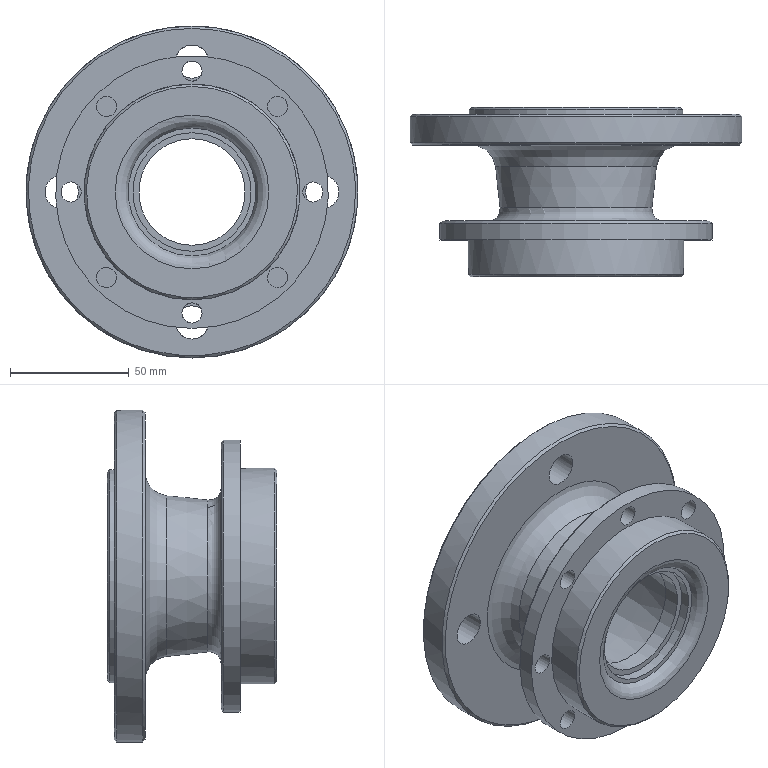Part | NX | features DATUM_CSYS 4, SKETCH 3, EXTRUDE 2, BLEND 1, CHAMFER 1, SWP104 1 | 1 solid | 37 faces | box 140 x 71.5 x 140 mm | volume 362768 mm3 | cylinder 19 | plane 8 | cone 7 | torus 3 | commonest cylinder face diameters 8.5 x8 14 x4 45 x1 50 x1 54 x1 90 x1
STEP:
#1=CARTESIAN_POINT('',(0.,0.,32.408));
#2=VERTEX_POINT('',#1);
#3=CARTESIAN_POINT('',(0.,0.,0.));
#4=DIRECTION('',(0.,1.,0.));
#5=DIRECTION('',(0.,0.,1.));
#6=AXIS2_PLACEMENT_3D('',#3,#4,#5);
#7=CIRCLE('',#6,32.408);
#8=EDGE_CURVE('',#2,#2,#7,.T.);
#9=ORIENTED_EDGE('',*,*,#8,.T.);
#10=EDGE_LOOP('',(#9));
#11=FACE_BOUND('',#10,.T.);
#12=CARTESIAN_POINT('',(0.,0.,44.5));
#13=VERTEX_POINT('',#12);
#14=CARTESIAN_POINT('',(0.,0.,0.));
#15=DIRECTION('',(0.,1.,0.));
#16=DIRECTION('',(0.,0.,1.));
#17=AXIS2_PLACEMENT_3D('',#14,#15,#16);
#18=CIRCLE('',#17,44.5);
#19=EDGE_CURVE('',#13,#13,#18,.F.);
#20=ORIENTED_EDGE('',*,*,#19,.T.);
#21=EDGE_LOOP('',(#20));
#22=FACE_BOUND('',#21,.T.);
#23=CARTESIAN_POINT('',(0.,0.,45.5));
#24=DIRECTION('',(0.,1.,0.));
#25=DIRECTION('',(0.,0.,1.));
#26=AXIS2_PLACEMENT_3D('',#23,#24,#25);
#27=PLANE('',#26);
#28=ADVANCED_FACE('',(#11,#22),#27,.F.);
#29=CARTESIAN_POINT('',(0.,4.5,-25.));
#30=VERTEX_POINT('',#29);
#31=CARTESIAN_POINT('',(0.,4.5,0.));
#32=DIRECTION('',(0.,-1.,0.));
#33=DIRECTION('',(0.,0.,-1.));
#34=AXIS2_PLACEMENT_3D('',#31,#32,#33);
#35=CIRCLE('',#34,25.);
#36=EDGE_CURVE('',#30,#30,#35,.T.);
#37=ORIENTED_EDGE('',*,*,#36,.F.);
#38=EDGE_LOOP('',(#37));
#39=FACE_BOUND('',#38,.T.);
#40=CARTESIAN_POINT('',(0.,4.5,-27.));
#41=VERTEX_POINT('',#40);
#42=CARTESIAN_POINT('',(0.,4.5,0.));
#43=DIRECTION('',(0.,-1.,0.));
#44=DIRECTION('',(0.,0.,-1.));
#45=AXIS2_PLACEMENT_3D('',#42,#43,#44);
#46=CIRCLE('',#45,27.);
#47=EDGE_CURVE('',#41,#41,#46,.T.);
#48=ORIENTED_EDGE('',*,*,#47,.T.);
#49=EDGE_LOOP('',(#48));
#50=FACE_BOUND('',#49,.T.);
#51=CARTESIAN_POINT('',(0.,4.5,27.));
#52=DIRECTION('',(0.,1.,0.));
#53=DIRECTION('',(0.,0.,1.));
#54=AXIS2_PLACEMENT_3D('',#51,#52,#53);
#55=PLANE('',#54);
#56=ADVANCED_FACE('',(#39,#50),#55,.F.);
#57=CARTESIAN_POINT('',(0.,8.5,-25.));
#58=VERTEX_POINT('',#57);
#59=CARTESIAN_POINT('',(0.,8.5,0.));
#60=DIRECTION('',(0.,-1.,0.));
#61=DIRECTION('',(0.,0.,-1.));
#62=AXIS2_PLACEMENT_3D('',#59,#60,#61);
#63=CIRCLE('',#62,25.);
#64=EDGE_CURVE('',#58,#58,#63,.T.);
#65=ORIENTED_EDGE('',*,*,#64,.F.);
#66=EDGE_LOOP('',(#65));
#67=FACE_BOUND('',#66,.T.);
#68=ORIENTED_EDGE('',*,*,#36,.T.);
#69=EDGE_LOOP('',(#68));
#70=FACE_BOUND('',#69,.T.);
#71=CARTESIAN_POINT('',(0.,0.,0.));
#72=DIRECTION('',(0.,-1.,0.));
#73=DIRECTION('',(0.,0.,-1.));
#74=AXIS2_PLACEMENT_3D('',#71,#72,#73);
#75=CYLINDRICAL_SURFACE('',#74,25.);
#76=ADVANCED_FACE('',(#67,#70),#75,.F.);
#77=CARTESIAN_POINT('',(0.,8.5,-22.5));
#78=VERTEX_POINT('',#77);
#79=CARTESIAN_POINT('',(0.,8.5,0.));
#80=DIRECTION('',(0.,-1.,0.));
#81=DIRECTION('',(0.,0.,-1.));
#82=AXIS2_PLACEMENT_3D('',#79,#80,#81);
#83=CIRCLE('',#82,22.5);
#84=EDGE_CURVE('',#78,#78,#83,.T.);
#85=ORIENTED_EDGE('',*,*,#84,.F.);
#86=EDGE_LOOP('',(#85));
#87=FACE_BOUND('',#86,.T.);
#88=ORIENTED_EDGE('',*,*,#64,.T.);
#89=EDGE_LOOP('',(#88));
#90=FACE_BOUND('',#89,.T.);
#91=CARTESIAN_POINT('',(0.,8.5,25.));
#92=DIRECTION('',(0.,1.,0.));
#93=DIRECTION('',(0.,0.,1.));
#94=AXIS2_PLACEMENT_3D('',#91,#92,#93);
#95=PLANE('',#94);
#96=ADVANCED_FACE('',(#87,#90),#95,.F.);
#97=CARTESIAN_POINT('',(0.,15.5,-22.5));
#98=VERTEX_POINT('',#97);
#99=CARTESIAN_POINT('',(0.,15.5,0.));
#100=DIRECTION('',(0.,-1.,0.));
#101=DIRECTION('',(0.,0.,-1.));
#102=AXIS2_PLACEMENT_3D('',#99,#100,#101);
#103=CIRCLE('',#102,22.5);
#104=EDGE_CURVE('',#98,#98,#103,.T.);
#105=ORIENTED_EDGE('',*,*,#104,.F.);
#106=EDGE_LOOP('',(#105));
#107=FACE_BOUND('',#106,.T.);
#108=ORIENTED_EDGE('',*,*,#84,.T.);
#109=EDGE_LOOP('',(#108));
#110=FACE_BOUND('',#109,.T.);
#111=CARTESIAN_POINT('',(0.,0.,0.));
#112=DIRECTION('',(0.,-1.,0.));
#113=DIRECTION('',(0.,0.,-1.));
#114=AXIS2_PLACEMENT_3D('',#111,#112,#113);
#115=CYLINDRICAL_SURFACE('',#114,22.5);
#116=ADVANCED_FACE('',(#107,#110),#115,.F.);
#117=CARTESIAN_POINT('',(0.,56.5,-27.));
#118=VERTEX_POINT('',#117);
#119=CARTESIAN_POINT('',(0.,56.5,0.));
#120=DIRECTION('',(0.,-1.,0.));
#121=DIRECTION('',(0.,0.,-1.));
#122=AXIS2_PLACEMENT_3D('',#119,#120,#121);
#123=CIRCLE('',#122,27.);
#124=EDGE_CURVE('',#118,#118,#123,.T.);
#125=ORIENTED_EDGE('',*,*,#124,.F.);
#126=EDGE_LOOP('',(#125));
#127=FACE_BOUND('',#126,.T.);
#128=ORIENTED_EDGE('',*,*,#104,.T.);
#129=EDGE_LOOP('',(#128));
#130=FACE_BOUND('',#129,.T.);
#131=CARTESIAN_POINT('',(0.,15.5,0.));
#132=DIRECTION('',(0.,1.,0.));
#133=DIRECTION('',(0.,0.,1.));
#134=AXIS2_PLACEMENT_3D('',#131,#132,#133);
#135=CONICAL_SURFACE('',#134,22.5,0.1093);
#136=ADVANCED_FACE('',(#127,#130),#135,.F.);
#137=CARTESIAN_POINT('',(0.,71.5,-27.));
#138=VERTEX_POINT('',#137);
#139=CARTESIAN_POINT('',(0.,71.5,0.));
#140=DIRECTION('',(0.,-1.,0.));
#141=DIRECTION('',(0.,0.,-1.));
#142=AXIS2_PLACEMENT_3D('',#139,#140,#141);
#143=CIRCLE('',#142,27.);
#144=EDGE_CURVE('',#138,#138,#143,.T.);
#145=ORIENTED_EDGE('',*,*,#144,.F.);
#146=EDGE_LOOP('',(#145));
#147=FACE_BOUND('',#146,.T.);
#148=ORIENTED_EDGE('',*,*,#124,.T.);
#149=EDGE_LOOP('',(#148));
#150=FACE_BOUND('',#149,.T.);
#151=CARTESIAN_POINT('',(0.,0.,0.));
#152=DIRECTION('',(0.,-1.,0.));
#153=DIRECTION('',(0.,0.,-1.));
#154=AXIS2_PLACEMENT_3D('',#151,#152,#153);
#155=CYLINDRICAL_SURFACE('',#154,27.);
#156=ADVANCED_FACE('',(#147,#150),#155,.F.);
#157=CARTESIAN_POINT('',(0.,71.5,-44.));
#158=VERTEX_POINT('',#157);
#159=CARTESIAN_POINT('',(0.,71.5,0.));
#160=DIRECTION('',(0.,-1.,0.));
#161=DIRECTION('',(0.,0.,-1.));
#162=AXIS2_PLACEMENT_3D('',#159,#160,#161);
#163=CIRCLE('',#162,44.);
#164=EDGE_CURVE('',#158,#158,#163,.F.);
#165=ORIENTED_EDGE('',*,*,#164,.T.);
#166=EDGE_LOOP('',(#165));
#167=FACE_BOUND('',#166,.T.);
#168=ORIENTED_EDGE('',*,*,#144,.T.);
#169=EDGE_LOOP('',(#168));
#170=FACE_BOUND('',#169,.T.);
#171=CARTESIAN_POINT('',(0.,71.5,27.));
#172=DIRECTION('',(0.,-1.,0.));
#173=DIRECTION('',(0.,0.,-1.));
#174=AXIS2_PLACEMENT_3D('',#171,#172,#173);
#175=PLANE('',#174);
#176=ADVANCED_FACE('',(#167,#170),#175,.F.);
#177=CARTESIAN_POINT('',(0.,70.5,-45.));
#178=VERTEX_POINT('',#177);
#179=CARTESIAN_POINT('',(0.,70.5,0.));
#180=DIRECTION('',(0.,-1.,0.));
#181=DIRECTION('',(0.,0.,-1.));
#182=AXIS2_PLACEMENT_3D('',#179,#180,#181);
#183=CIRCLE('',#182,45.);
#184=EDGE_CURVE('',#178,#178,#183,.T.);
#185=ORIENTED_EDGE('',*,*,#184,.T.);
#186=EDGE_LOOP('',(#185));
#187=FACE_BOUND('',#186,.T.);
#188=CARTESIAN_POINT('',(0.,68.5,-45.));
#189=VERTEX_POINT('',#188);
#190=CARTESIAN_POINT('',(0.,68.5,0.));
#191=DIRECTION('',(0.,-1.,0.));
#192=DIRECTION('',(0.,0.,-1.));
#193=AXIS2_PLACEMENT_3D('',#190,#191,#192);
#194=CIRCLE('',#193,45.);
#195=EDGE_CURVE('',#189,#189,#194,.T.);
#196=ORIENTED_EDGE('',*,*,#195,.F.);
#197=EDGE_LOOP('',(#196));
#198=FACE_BOUND('',#197,.T.);
#199=CARTESIAN_POINT('',(0.,0.,0.));
#200=DIRECTION('',(0.,-1.,0.));
#201=DIRECTION('',(0.,0.,-1.));
#202=AXIS2_PLACEMENT_3D('',#199,#200,#201);
#203=CYLINDRICAL_SURFACE('',#202,45.);
#204=ADVANCED_FACE('',(#187,#198),#203,.T.);
#205=CARTESIAN_POINT('',(55.,68.5,-7.));
#206=VERTEX_POINT('',#205);
#207=CARTESIAN_POINT('',(55.,68.5,0.));
#208=DIRECTION('',(0.,-1.,0.));
#209=DIRECTION('',(0.,0.,-1.));
#210=AXIS2_PLACEMENT_3D('',#207,#208,#209);
#211=CIRCLE('',#210,7.);
#212=EDGE_CURVE('',#206,#206,#211,.T.);
#213=ORIENTED_EDGE('',*,*,#212,.T.);
#214=EDGE_LOOP('',(#213));
#215=FACE_BOUND('',#214,.T.);
#216=CARTESIAN_POINT('',(0.,68.5,-62.));
#217=VERTEX_POINT('',#216);
#218=CARTESIAN_POINT('',(0.,68.5,-55.));
#219=DIRECTION('',(0.,-1.,0.));
#220=DIRECTION('',(0.,0.,-1.));
#221=AXIS2_PLACEMENT_3D('',#218,#219,#220);
#222=CIRCLE('',#221,7.);
#223=EDGE_CURVE('',#217,#217,#222,.T.);
#224=ORIENTED_EDGE('',*,*,#223,.T.);
#225=EDGE_LOOP('',(#224));
#226=FACE_BOUND('',#225,.T.);
#227=CARTESIAN_POINT('',(-55.,68.5,-7.));
#228=VERTEX_POINT('',#227);
#229=CARTESIAN_POINT('',(-55.,68.5,0.));
#230=DIRECTION('',(0.,-1.,0.));
#231=DIRECTION('',(0.,0.,-1.));
#232=AXIS2_PLACEMENT_3D('',#229,#230,#231);
#233=CIRCLE('',#232,7.);
#234=EDGE_CURVE('',#228,#228,#233,.T.);
#235=ORIENTED_EDGE('',*,*,#234,.T.);
#236=EDGE_LOOP('',(#235));
#237=FACE_BOUND('',#236,.T.);
#238=CARTESIAN_POINT('',(0.,68.5,48.));
#239=VERTEX_POINT('',#238);
#240=CARTESIAN_POINT('',(0.,68.5,55.));
#241=DIRECTION('',(0.,-1.,0.));
#242=DIRECTION('',(0.,0.,-1.));
#243=AXIS2_PLACEMENT_3D('',#240,#241,#242);
#244=CIRCLE('',#243,7.);
#245=EDGE_CURVE('',#239,#239,#244,.T.);
#246=ORIENTED_EDGE('',*,*,#245,.T.);
#247=EDGE_LOOP('',(#246));
#248=FACE_BOUND('',#247,.T.);
#249=CARTESIAN_POINT('',(0.,68.5,-69.));
#250=VERTEX_POINT('',#249);
#251=CARTESIAN_POINT('',(0.,68.5,0.));
#252=DIRECTION('',(0.,-1.,0.));
#253=DIRECTION('',(0.,0.,-1.));
#254=AXIS2_PLACEMENT_3D('',#251,#252,#253);
#255=CIRCLE('',#254,69.);
#256=EDGE_CURVE('',#250,#250,#255,.F.);
#257=ORIENTED_EDGE('',*,*,#256,.T.);
#258=EDGE_LOOP('',(#257));
#259=FACE_BOUND('',#258,.T.);
#260=ORIENTED_EDGE('',*,*,#195,.T.);
#261=EDGE_LOOP('',(#260));
#262=FACE_BOUND('',#261,.T.);
#263=CARTESIAN_POINT('',(0.,68.5,45.));
#264=DIRECTION('',(0.,-1.,0.));
#265=DIRECTION('',(0.,0.,-1.));
#266=AXIS2_PLACEMENT_3D('',#263,#264,#265);
#267=PLANE('',#266);
#268=ADVANCED_FACE('',(#215,#226,#237,#248,#259,#262),#267,.F.);
#269=CARTESIAN_POINT('',(0.,67.5,-70.));
#270=VERTEX_POINT('',#269);
#271=CARTESIAN_POINT('',(0.,67.5,0.));
#272=DIRECTION('',(0.,-1.,0.));
#273=DIRECTION('',(0.,0.,-1.));
#274=AXIS2_PLACEMENT_3D('',#271,#272,#273);
#275=CIRCLE('',#274,70.);
#276=EDGE_CURVE('',#270,#270,#275,.T.);
#277=ORIENTED_EDGE('',*,*,#276,.T.);
#278=EDGE_LOOP('',(#277));
#279=FACE_BOUND('',#278,.T.);
#280=CARTESIAN_POINT('',(0.,56.5,70.));
#281=VERTEX_POINT('',#280);
#282=CARTESIAN_POINT('',(0.,56.5,0.));
#283=DIRECTION('',(0.,1.,0.));
#284=DIRECTION('',(0.,0.,1.));
#285=AXIS2_PLACEMENT_3D('',#282,#283,#284);
#286=CIRCLE('',#285,70.);
#287=EDGE_CURVE('',#281,#281,#286,.T.);
#288=ORIENTED_EDGE('',*,*,#287,.T.);
#289=EDGE_LOOP('',(#288));
#290=FACE_BOUND('',#289,.T.);
#291=CARTESIAN_POINT('',(0.,0.,0.));
#292=DIRECTION('',(0.,-1.,0.));
#293=DIRECTION('',(0.,0.,-1.));
#294=AXIS2_PLACEMENT_3D('',#291,#292,#293);
#295=CYLINDRICAL_SURFACE('',#294,70.);
#296=ADVANCED_FACE('',(#279,#290),#295,.T.);
#297=CARTESIAN_POINT('',(55.,55.5,-7.));
#298=VERTEX_POINT('',#297);
#299=CARTESIAN_POINT('',(55.,55.5,0.));
#300=DIRECTION('',(0.,-1.,0.));
#301=DIRECTION('',(0.,0.,-1.));
#302=AXIS2_PLACEMENT_3D('',#299,#300,#301);
#303=CIRCLE('',#302,7.);
#304=EDGE_CURVE('',#298,#298,#303,.T.);
#305=ORIENTED_EDGE('',*,*,#304,.F.);
#306=EDGE_LOOP('',(#305));
#307=FACE_BOUND('',#306,.T.);
#308=CARTESIAN_POINT('',(-7.,55.5,-55.));
#309=VERTEX_POINT('',#308);
#310=CARTESIAN_POINT('',(0.,55.5,-55.));
#311=DIRECTION('',(0.,-1.,0.));
#312=DIRECTION('',(-1.,0.,0.));
#313=AXIS2_PLACEMENT_3D('',#310,#311,#312);
#314=CIRCLE('',#313,7.);
#315=EDGE_CURVE('',#309,#309,#314,.T.);
#316=ORIENTED_EDGE('',*,*,#315,.F.);
#317=EDGE_LOOP('',(#316));
#318=FACE_BOUND('',#317,.T.);
#319=CARTESIAN_POINT('',(-55.,55.5,7.));
#320=VERTEX_POINT('',#319);
#321=CARTESIAN_POINT('',(-55.,55.5,0.));
#322=DIRECTION('',(0.,-1.,0.));
#323=DIRECTION('',(0.,0.,1.));
#324=AXIS2_PLACEMENT_3D('',#321,#322,#323);
#325=CIRCLE('',#324,7.);
#326=EDGE_CURVE('',#320,#320,#325,.T.);
#327=ORIENTED_EDGE('',*,*,#326,.F.);
#328=EDGE_LOOP('',(#327));
#329=FACE_BOUND('',#328,.T.);
#330=CARTESIAN_POINT('',(7.,55.5,55.));
#331=VERTEX_POINT('',#330);
#332=CARTESIAN_POINT('',(0.,55.5,55.));
#333=DIRECTION('',(0.,-1.,0.));
#334=DIRECTION('',(1.,0.,0.));
#335=AXIS2_PLACEMENT_3D('',#332,#333,#334);
#336=CIRCLE('',#335,7.);
#337=EDGE_CURVE('',#331,#331,#336,.T.);
#338=ORIENTED_EDGE('',*,*,#337,.F.);
#339=EDGE_LOOP('',(#338));
#340=FACE_BOUND('',#339,.T.);
#341=CARTESIAN_POINT('',(0.,55.5,69.));
#342=VERTEX_POINT('',#341);
#343=CARTESIAN_POINT('',(0.,55.5,0.));
#344=DIRECTION('',(0.,1.,0.));
#345=DIRECTION('',(0.,0.,1.));
#346=AXIS2_PLACEMENT_3D('',#343,#344,#345);
#347=CIRCLE('',#346,69.);
#348=EDGE_CURVE('',#342,#342,#347,.F.);
#349=ORIENTED_EDGE('',*,*,#348,.T.);
#350=EDGE_LOOP('',(#349));
#351=FACE_BOUND('',#350,.T.);
#352=CARTESIAN_POINT('',(0.,55.5,-43.901));
#353=VERTEX_POINT('',#352);
#354=CARTESIAN_POINT('',(0.,55.5,0.));
#355=DIRECTION('',(0.,-1.,0.));
#356=DIRECTION('',(0.,0.,-1.));
#357=AXIS2_PLACEMENT_3D('',#354,#355,#356);
#358=CIRCLE('',#357,43.901);
#359=EDGE_CURVE('',#353,#353,#358,.T.);
#360=ORIENTED_EDGE('',*,*,#359,.F.);
#361=EDGE_LOOP('',(#360));
#362=FACE_BOUND('',#361,.T.);
#363=CARTESIAN_POINT('',(0.,55.5,70.));
#364=DIRECTION('',(0.,1.,0.));
#365=DIRECTION('',(0.,0.,1.));
#366=AXIS2_PLACEMENT_3D('',#363,#364,#365);
#367=PLANE('',#366);
#368=ADVANCED_FACE('',(#307,#318,#329,#340,#351,#362),#367,.F.);
#369=CARTESIAN_POINT('',(0.,46.591,-33.96));
#370=VERTEX_POINT('',#369);
#371=CARTESIAN_POINT('',(0.,46.591,0.));
#372=DIRECTION('',(0.,-1.,0.));
#373=DIRECTION('',(0.,0.,-1.));
#374=AXIS2_PLACEMENT_3D('',#371,#372,#373);
#375=CIRCLE('',#374,33.96);
#376=EDGE_CURVE('',#370,#370,#375,.T.);
#377=ORIENTED_EDGE('',*,*,#376,.F.);
#378=EDGE_LOOP('',(#377));
#379=FACE_BOUND('',#378,.T.);
#380=ORIENTED_EDGE('',*,*,#359,.T.);
#381=EDGE_LOOP('',(#380));
#382=FACE_BOUND('',#381,.T.);
#383=CARTESIAN_POINT('',(0.,45.5,0.));
#384=DIRECTION('',(0.,-1.,0.));
#385=DIRECTION('',(0.,0.,-1.));
#386=AXIS2_PLACEMENT_3D('',#383,#384,#385);
#387=TOROIDAL_SURFACE('',#386,43.901,10.);
#388=ADVANCED_FACE('',(#379,#382),#387,.F.);
#389=CARTESIAN_POINT('',(0.,29.046,-32.035));
#390=VERTEX_POINT('',#389);
#391=CARTESIAN_POINT('',(0.,29.046,0.));
#392=DIRECTION('',(0.,-1.,0.));
#393=DIRECTION('',(0.,0.,-1.));
#394=AXIS2_PLACEMENT_3D('',#391,#392,#393);
#395=CIRCLE('',#394,32.035);
#396=EDGE_CURVE('',#390,#390,#395,.T.);
#397=ORIENTED_EDGE('',*,*,#396,.F.);
#398=EDGE_LOOP('',(#397));
#399=FACE_BOUND('',#398,.T.);
#400=ORIENTED_EDGE('',*,*,#376,.T.);
#401=EDGE_LOOP('',(#400));
#402=FACE_BOUND('',#401,.T.);
#403=CARTESIAN_POINT('',(0.,46.591,0.));
#404=DIRECTION('',(0.,1.,0.));
#405=DIRECTION('',(0.,0.,1.));
#406=AXIS2_PLACEMENT_3D('',#403,#404,#405);
#407=CONICAL_SURFACE('',#406,33.96,0.1093);
#408=ADVANCED_FACE('',(#399,#402),#407,.T.);
#409=CARTESIAN_POINT('',(0.,23.5,-37.005));
#410=VERTEX_POINT('',#409);
#411=CARTESIAN_POINT('',(0.,23.5,0.));
#412=DIRECTION('',(0.,-1.,0.));
#413=DIRECTION('',(0.,0.,-1.));
#414=AXIS2_PLACEMENT_3D('',#411,#412,#413);
#415=CIRCLE('',#414,37.005);
#416=EDGE_CURVE('',#410,#410,#415,.T.);
#417=ORIENTED_EDGE('',*,*,#416,.F.);
#418=EDGE_LOOP('',(#417));
#419=FACE_BOUND('',#418,.T.);
#420=ORIENTED_EDGE('',*,*,#396,.T.);
#421=EDGE_LOOP('',(#420));
#422=FACE_BOUND('',#421,.T.);
#423=CARTESIAN_POINT('',(0.,28.5,0.));
#424=DIRECTION('',(0.,-1.,0.));
#425=DIRECTION('',(0.,0.,-1.));
#426=AXIS2_PLACEMENT_3D('',#423,#424,#425);
#427=TOROIDAL_SURFACE('',#426,37.005,5.);
#428=ADVANCED_FACE('',(#419,#422),#427,.F.);
#429=CARTESIAN_POINT('',(51.,23.5,-4.25));
#430=VERTEX_POINT('',#429);
#431=CARTESIAN_POINT('',(51.,23.5,0.));
#432=DIRECTION('',(0.,-1.,0.));
#433=DIRECTION('',(0.,0.,-1.));
#434=AXIS2_PLACEMENT_3D('',#431,#432,#433);
#435=CIRCLE('',#434,4.25);
#436=EDGE_CURVE('',#430,#430,#435,.T.);
#437=ORIENTED_EDGE('',*,*,#436,.T.);
#438=EDGE_LOOP('',(#437));
#439=FACE_BOUND('',#438,.T.);
#440=CARTESIAN_POINT('',(36.062,23.5,-40.312));
#441=VERTEX_POINT('',#440);
#442=CARTESIAN_POINT('',(36.062,23.5,-36.062));
#443=DIRECTION('',(0.,-1.,0.));
#444=DIRECTION('',(0.,0.,-1.));
#445=AXIS2_PLACEMENT_3D('',#442,#443,#444);
#446=CIRCLE('',#445,4.25);
#447=EDGE_CURVE('',#441,#441,#446,.T.);
#448=ORIENTED_EDGE('',*,*,#447,.T.);
#449=EDGE_LOOP('',(#448));
#450=FACE_BOUND('',#449,.T.);
#451=CARTESIAN_POINT('',(0.,23.5,-55.25));
#452=VERTEX_POINT('',#451);
#453=CARTESIAN_POINT('',(0.,23.5,-51.));
#454=DIRECTION('',(0.,-1.,0.));
#455=DIRECTION('',(0.,0.,-1.));
#456=AXIS2_PLACEMENT_3D('',#453,#454,#455);
#457=CIRCLE('',#456,4.25);
#458=EDGE_CURVE('',#452,#452,#457,.T.);
#459=ORIENTED_EDGE('',*,*,#458,.T.);
#460=EDGE_LOOP('',(#459));
#461=FACE_BOUND('',#460,.T.);
#462=CARTESIAN_POINT('',(-36.062,23.5,-40.312));
#463=VERTEX_POINT('',#462);
#464=CARTESIAN_POINT('',(-36.062,23.5,-36.062));
#465=DIRECTION('',(0.,-1.,0.));
#466=DIRECTION('',(0.,0.,-1.));
#467=AXIS2_PLACEMENT_3D('',#464,#465,#466);
#468=CIRCLE('',#467,4.25);
#469=EDGE_CURVE('',#463,#463,#468,.T.);
#470=ORIENTED_EDGE('',*,*,#469,.T.);
#471=EDGE_LOOP('',(#470));
#472=FACE_BOUND('',#471,.T.);
#473=CARTESIAN_POINT('',(-51.,23.5,-4.25));
#474=VERTEX_POINT('',#473);
#475=CARTESIAN_POINT('',(-51.,23.5,0.));
#476=DIRECTION('',(0.,-1.,0.));
#477=DIRECTION('',(0.,0.,-1.));
#478=AXIS2_PLACEMENT_3D('',#475,#476,#477);
#479=CIRCLE('',#478,4.25);
#480=EDGE_CURVE('',#474,#474,#479,.T.);
#481=ORIENTED_EDGE('',*,*,#480,.T.);
#482=EDGE_LOOP('',(#481));
#483=FACE_BOUND('',#482,.T.);
#484=CARTESIAN_POINT('',(-36.062,23.5,31.812));
#485=VERTEX_POINT('',#484);
#486=CARTESIAN_POINT('',(-36.062,23.5,36.062));
#487=DIRECTION('',(0.,-1.,0.));
#488=DIRECTION('',(0.,0.,-1.));
#489=AXIS2_PLACEMENT_3D('',#486,#487,#488);
#490=CIRCLE('',#489,4.25);
#491=EDGE_CURVE('',#485,#485,#490,.T.);
#492=ORIENTED_EDGE('',*,*,#491,.T.);
#493=EDGE_LOOP('',(#492));
#494=FACE_BOUND('',#493,.T.);
#495=CARTESIAN_POINT('',(0.,23.5,46.75));
#496=VERTEX_POINT('',#495);
#497=CARTESIAN_POINT('',(0.,23.5,51.));
#498=DIRECTION('',(0.,-1.,0.));
#499=DIRECTION('',(0.,0.,-1.));
#500=AXIS2_PLACEMENT_3D('',#497,#498,#499);
#501=CIRCLE('',#500,4.25);
#502=EDGE_CURVE('',#496,#496,#501,.T.);
#503=ORIENTED_EDGE('',*,*,#502,.T.);
#504=EDGE_LOOP('',(#503));
#505=FACE_BOUND('',#504,.T.);
#506=CARTESIAN_POINT('',(36.062,23.5,31.812));
#507=VERTEX_POINT('',#506);
#508=CARTESIAN_POINT('',(36.062,23.5,36.062));
#509=DIRECTION('',(0.,-1.,0.));
#510=DIRECTION('',(0.,0.,-1.));
#511=AXIS2_PLACEMENT_3D('',#508,#509,#510);
#512=CIRCLE('',#511,4.25);
#513=EDGE_CURVE('',#507,#507,#512,.T.);
#514=ORIENTED_EDGE('',*,*,#513,.T.);
#515=EDGE_LOOP('',(#514));
#516=FACE_BOUND('',#515,.T.);
#517=CARTESIAN_POINT('',(0.,23.5,-56.5));
#518=VERTEX_POINT('',#517);
#519=CARTESIAN_POINT('',(0.,23.5,0.));
#520=DIRECTION('',(0.,-1.,0.));
#521=DIRECTION('',(0.,0.,-1.));
#522=AXIS2_PLACEMENT_3D('',#519,#520,#521);
#523=CIRCLE('',#522,56.5);
#524=EDGE_CURVE('',#518,#518,#523,.F.);
#525=ORIENTED_EDGE('',*,*,#524,.T.);
#526=EDGE_LOOP('',(#525));
#527=FACE_BOUND('',#526,.T.);
#528=ORIENTED_EDGE('',*,*,#416,.T.);
#529=EDGE_LOOP('',(#528));
#530=FACE_BOUND('',#529,.T.);
#531=CARTESIAN_POINT('',(0.,23.5,37.005));
#532=DIRECTION('',(0.,-1.,0.));
#533=DIRECTION('',(0.,0.,-1.));
#534=AXIS2_PLACEMENT_3D('',#531,#532,#533);
#535=PLANE('',#534);
#536=ADVANCED_FACE('',(#439,#450,#461,#472,#483,#494,#505,#516,#527,#530),#535,.F.);
#537=CARTESIAN_POINT('',(0.,22.5,-57.5));
#538=VERTEX_POINT('',#537);
#539=CARTESIAN_POINT('',(0.,22.5,0.));
#540=DIRECTION('',(0.,-1.,0.));
#541=DIRECTION('',(0.,0.,-1.));
#542=AXIS2_PLACEMENT_3D('',#539,#540,#541);
#543=CIRCLE('',#542,57.5);
#544=EDGE_CURVE('',#538,#538,#543,.T.);
#545=ORIENTED_EDGE('',*,*,#544,.T.);
#546=EDGE_LOOP('',(#545));
#547=FACE_BOUND('',#546,.T.);
#548=CARTESIAN_POINT('',(0.,15.5,-57.5));
#549=VERTEX_POINT('',#548);
#550=CARTESIAN_POINT('',(0.,15.5,0.));
#551=DIRECTION('',(0.,-1.,0.));
#552=DIRECTION('',(0.,0.,-1.));
#553=AXIS2_PLACEMENT_3D('',#550,#551,#552);
#554=CIRCLE('',#553,57.5);
#555=EDGE_CURVE('',#549,#549,#554,.T.);
#556=ORIENTED_EDGE('',*,*,#555,.F.);
#557=EDGE_LOOP('',(#556));
#558=FACE_BOUND('',#557,.T.);
#559=CARTESIAN_POINT('',(0.,0.,0.));
#560=DIRECTION('',(0.,-1.,0.));
#561=DIRECTION('',(0.,0.,-1.));
#562=AXIS2_PLACEMENT_3D('',#559,#560,#561);
#563=CYLINDRICAL_SURFACE('',#562,57.5);
#564=ADVANCED_FACE('',(#547,#558),#563,.T.);
#565=CARTESIAN_POINT('',(51.,15.5,-4.25));
#566=VERTEX_POINT('',#565);
#567=CARTESIAN_POINT('',(51.,15.5,0.));
#568=DIRECTION('',(0.,-1.,0.));
#569=DIRECTION('',(0.,0.,-1.));
#570=AXIS2_PLACEMENT_3D('',#567,#568,#569);
#571=CIRCLE('',#570,4.25);
#572=EDGE_CURVE('',#566,#566,#571,.T.);
#573=ORIENTED_EDGE('',*,*,#572,.F.);
#574=EDGE_LOOP('',(#573));
#575=FACE_BOUND('',#574,.T.);
#576=CARTESIAN_POINT('',(33.057,15.5,-39.068));
#577=VERTEX_POINT('',#576);
#578=CARTESIAN_POINT('',(36.062,15.5,-36.062));
#579=DIRECTION('',(0.,-1.,0.));
#580=DIRECTION('',(-0.7071,0.,-0.7071));
#581=AXIS2_PLACEMENT_3D('',#578,#579,#580);
#582=CIRCLE('',#581,4.25);
#583=EDGE_CURVE('',#577,#577,#582,.T.);
#584=ORIENTED_EDGE('',*,*,#583,.F.);
#585=EDGE_LOOP('',(#584));
#586=FACE_BOUND('',#585,.T.);
#587=CARTESIAN_POINT('',(-4.25,15.5,-51.));
#588=VERTEX_POINT('',#587);
#589=CARTESIAN_POINT('',(0.,15.5,-51.));
#590=DIRECTION('',(0.,-1.,0.));
#591=DIRECTION('',(-1.,0.,0.));
#592=AXIS2_PLACEMENT_3D('',#589,#590,#591);
#593=CIRCLE('',#592,4.25);
#594=EDGE_CURVE('',#588,#588,#593,.T.);
#595=ORIENTED_EDGE('',*,*,#594,.F.);
#596=EDGE_LOOP('',(#595));
#597=FACE_BOUND('',#596,.T.);
#598=CARTESIAN_POINT('',(-39.068,15.5,-33.057));
#599=VERTEX_POINT('',#598);
#600=CARTESIAN_POINT('',(-36.062,15.5,-36.062));
#601=DIRECTION('',(0.,-1.,0.));
#602=DIRECTION('',(-0.7071,0.,0.7071));
#603=AXIS2_PLACEMENT_3D('',#600,#601,#602);
#604=CIRCLE('',#603,4.25);
#605=EDGE_CURVE('',#599,#599,#604,.T.);
#606=ORIENTED_EDGE('',*,*,#605,.F.);
#607=EDGE_LOOP('',(#606));
#608=FACE_BOUND('',#607,.T.);
#609=CARTESIAN_POINT('',(-51.,15.5,4.25));
#610=VERTEX_POINT('',#609);
#611=CARTESIAN_POINT('',(-51.,15.5,0.));
#612=DIRECTION('',(0.,-1.,0.));
#613=DIRECTION('',(0.,0.,1.));
#614=AXIS2_PLACEMENT_3D('',#611,#612,#613);
#615=CIRCLE('',#614,4.25);
#616=EDGE_CURVE('',#610,#610,#615,.T.);
#617=ORIENTED_EDGE('',*,*,#616,.F.);
#618=EDGE_LOOP('',(#617));
#619=FACE_BOUND('',#618,.T.);
#620=CARTESIAN_POINT('',(-33.057,15.5,39.068));
#621=VERTEX_POINT('',#620);
#622=CARTESIAN_POINT('',(-36.062,15.5,36.062));
#623=DIRECTION('',(0.,-1.,0.));
#624=DIRECTION('',(0.7071,0.,0.7071));
#625=AXIS2_PLACEMENT_3D('',#622,#623,#624);
#626=CIRCLE('',#625,4.25);
#627=EDGE_CURVE('',#621,#621,#626,.T.);
#628=ORIENTED_EDGE('',*,*,#627,.F.);
#629=EDGE_LOOP('',(#628));
#630=FACE_BOUND('',#629,.T.);
#631=CARTESIAN_POINT('',(4.25,15.5,51.));
#632=VERTEX_POINT('',#631);
#633=CARTESIAN_POINT('',(0.,15.5,51.));
#634=DIRECTION('',(0.,-1.,0.));
#635=DIRECTION('',(1.,0.,0.));
#636=AXIS2_PLACEMENT_3D('',#633,#634,#635);
#637=CIRCLE('',#636,4.25);
#638=EDGE_CURVE('',#632,#632,#637,.T.);
#639=ORIENTED_EDGE('',*,*,#638,.F.);
#640=EDGE_LOOP('',(#639));
#641=FACE_BOUND('',#640,.T.);
#642=CARTESIAN_POINT('',(39.068,15.5,33.057));
#643=VERTEX_POINT('',#642);
#644=CARTESIAN_POINT('',(36.062,15.5,36.062));
#645=DIRECTION('',(0.,-1.,0.));
#646=DIRECTION('',(0.7071,0.,-0.7071));
#647=AXIS2_PLACEMENT_3D('',#644,#645,#646);
#648=CIRCLE('',#647,4.25);
#649=EDGE_CURVE('',#643,#643,#648,.T.);
#650=ORIENTED_EDGE('',*,*,#649,.F.);
#651=EDGE_LOOP('',(#650));
#652=FACE_BOUND('',#651,.T.);
#653=CARTESIAN_POINT('',(0.,15.5,-45.5));
#654=VERTEX_POINT('',#653);
#655=CARTESIAN_POINT('',(0.,15.5,0.));
#656=DIRECTION('',(0.,-1.,0.));
#657=DIRECTION('',(0.,0.,-1.));
#658=AXIS2_PLACEMENT_3D('',#655,#656,#657);
#659=CIRCLE('',#658,45.5);
#660=EDGE_CURVE('',#654,#654,#659,.T.);
#661=ORIENTED_EDGE('',*,*,#660,.F.);
#662=EDGE_LOOP('',(#661));
#663=FACE_BOUND('',#662,.T.);
#664=ORIENTED_EDGE('',*,*,#555,.T.);
#665=EDGE_LOOP('',(#664));
#666=FACE_BOUND('',#665,.T.);
#667=CARTESIAN_POINT('',(0.,15.5,57.5));
#668=DIRECTION('',(0.,1.,0.));
#669=DIRECTION('',(0.,0.,1.));
#670=AXIS2_PLACEMENT_3D('',#667,#668,#669);
#671=PLANE('',#670);
#672=ADVANCED_FACE('',(#575,#586,#597,#608,#619,#630,#641,#652,#663,#666),#671,.F.);
#673=CARTESIAN_POINT('',(0.,1.,45.5));
#674=VERTEX_POINT('',#673);
#675=CARTESIAN_POINT('',(0.,1.,0.));
#676=DIRECTION('',(0.,1.,0.));
#677=DIRECTION('',(0.,0.,1.));
#678=AXIS2_PLACEMENT_3D('',#675,#676,#677);
#679=CIRCLE('',#678,45.5);
#680=EDGE_CURVE('',#674,#674,#679,.T.);
#681=ORIENTED_EDGE('',*,*,#680,.T.);
#682=EDGE_LOOP('',(#681));
#683=FACE_BOUND('',#682,.T.);
#684=ORIENTED_EDGE('',*,*,#660,.T.);
#685=EDGE_LOOP('',(#684));
#686=FACE_BOUND('',#685,.T.);
#687=CARTESIAN_POINT('',(0.,0.,0.));
#688=DIRECTION('',(0.,-1.,0.));
#689=DIRECTION('',(0.,0.,-1.));
#690=AXIS2_PLACEMENT_3D('',#687,#688,#689);
#691=CYLINDRICAL_SURFACE('',#690,45.5);
#692=ADVANCED_FACE('',(#683,#686),#691,.T.);
#693=ORIENTED_EDGE('',*,*,#164,.F.);
#694=EDGE_LOOP('',(#693));
#695=FACE_BOUND('',#694,.T.);
#696=ORIENTED_EDGE('',*,*,#184,.F.);
#697=EDGE_LOOP('',(#696));
#698=FACE_BOUND('',#697,.T.);
#699=CARTESIAN_POINT('',(0.,70.5,0.));
#700=DIRECTION('',(0.,-1.,0.));
#701=DIRECTION('',(0.,0.,-1.));
#702=AXIS2_PLACEMENT_3D('',#699,#700,#701);
#703=CONICAL_SURFACE('',#702,45.,0.7854);
#704=ADVANCED_FACE('',(#695,#698),#703,.T.);
#705=ORIENTED_EDGE('',*,*,#256,.F.);
#706=EDGE_LOOP('',(#705));
#707=FACE_BOUND('',#706,.T.);
#708=ORIENTED_EDGE('',*,*,#276,.F.);
#709=EDGE_LOOP('',(#708));
#710=FACE_BOUND('',#709,.T.);
#711=CARTESIAN_POINT('',(0.,67.5,0.));
#712=DIRECTION('',(0.,-1.,0.));
#713=DIRECTION('',(0.,0.,-1.));
#714=AXIS2_PLACEMENT_3D('',#711,#712,#713);
#715=CONICAL_SURFACE('',#714,70.,0.7854);
#716=ADVANCED_FACE('',(#707,#710),#715,.T.);
#717=ORIENTED_EDGE('',*,*,#287,.F.);
#718=EDGE_LOOP('',(#717));
#719=FACE_BOUND('',#718,.T.);
#720=ORIENTED_EDGE('',*,*,#348,.F.);
#721=EDGE_LOOP('',(#720));
#722=FACE_BOUND('',#721,.T.);
#723=CARTESIAN_POINT('',(0.,55.5,0.));
#724=DIRECTION('',(0.,1.,0.));
#725=DIRECTION('',(0.,0.,1.));
#726=AXIS2_PLACEMENT_3D('',#723,#724,#725);
#727=CONICAL_SURFACE('',#726,69.,0.7854);
#728=ADVANCED_FACE('',(#719,#722),#727,.T.);
#729=ORIENTED_EDGE('',*,*,#524,.F.);
#730=EDGE_LOOP('',(#729));
#731=FACE_BOUND('',#730,.T.);
#732=ORIENTED_EDGE('',*,*,#544,.F.);
#733=EDGE_LOOP('',(#732));
#734=FACE_BOUND('',#733,.T.);
#735=CARTESIAN_POINT('',(0.,22.5,0.));
#736=DIRECTION('',(0.,-1.,0.));
#737=DIRECTION('',(0.,0.,-1.));
#738=AXIS2_PLACEMENT_3D('',#735,#736,#737);
#739=CONICAL_SURFACE('',#738,57.5,0.7854);
#740=ADVANCED_FACE('',(#731,#734),#739,.T.);
#741=ORIENTED_EDGE('',*,*,#680,.F.);
#742=EDGE_LOOP('',(#741));
#743=FACE_BOUND('',#742,.T.);
#744=ORIENTED_EDGE('',*,*,#19,.F.);
#745=EDGE_LOOP('',(#744));
#746=FACE_BOUND('',#745,.T.);
#747=CARTESIAN_POINT('',(0.,0.,0.));
#748=DIRECTION('',(0.,1.,0.));
#749=DIRECTION('',(0.,0.,1.));
#750=AXIS2_PLACEMENT_3D('',#747,#748,#749);
#751=CONICAL_SURFACE('',#750,44.5,0.7854);
#752=ADVANCED_FACE('',(#743,#746),#751,.T.);
#753=ORIENTED_EDGE('',*,*,#649,.T.);
#754=EDGE_LOOP('',(#753));
#755=FACE_BOUND('',#754,.T.);
#756=ORIENTED_EDGE('',*,*,#513,.F.);
#757=EDGE_LOOP('',(#756));
#758=FACE_BOUND('',#757,.T.);
#759=CARTESIAN_POINT('',(36.062,37.5,36.062));
#760=DIRECTION('',(0.,-1.,0.));
#761=DIRECTION('',(0.,0.,-1.));
#762=AXIS2_PLACEMENT_3D('',#759,#760,#761);
#763=CYLINDRICAL_SURFACE('',#762,4.25);
#764=ADVANCED_FACE('',(#755,#758),#763,.F.);
#765=ORIENTED_EDGE('',*,*,#638,.T.);
#766=EDGE_LOOP('',(#765));
#767=FACE_BOUND('',#766,.T.);
#768=ORIENTED_EDGE('',*,*,#502,.F.);
#769=EDGE_LOOP('',(#768));
#770=FACE_BOUND('',#769,.T.);
#771=CARTESIAN_POINT('',(0.,37.5,51.));
#772=DIRECTION('',(0.,-1.,0.));
#773=DIRECTION('',(0.,0.,-1.));
#774=AXIS2_PLACEMENT_3D('',#771,#772,#773);
#775=CYLINDRICAL_SURFACE('',#774,4.25);
#776=ADVANCED_FACE('',(#767,#770),#775,.F.);
#777=ORIENTED_EDGE('',*,*,#627,.T.);
#778=EDGE_LOOP('',(#777));
#779=FACE_BOUND('',#778,.T.);
#780=ORIENTED_EDGE('',*,*,#491,.F.);
#781=EDGE_LOOP('',(#780));
#782=FACE_BOUND('',#781,.T.);
#783=CARTESIAN_POINT('',(-36.062,37.5,36.062));
#784=DIRECTION('',(0.,-1.,0.));
#785=DIRECTION('',(0.,0.,-1.));
#786=AXIS2_PLACEMENT_3D('',#783,#784,#785);
#787=CYLINDRICAL_SURFACE('',#786,4.25);
#788=ADVANCED_FACE('',(#779,#782),#787,.F.);
#789=ORIENTED_EDGE('',*,*,#616,.T.);
#790=EDGE_LOOP('',(#789));
#791=FACE_BOUND('',#790,.T.);
#792=ORIENTED_EDGE('',*,*,#480,.F.);
#793=EDGE_LOOP('',(#792));
#794=FACE_BOUND('',#793,.T.);
#795=CARTESIAN_POINT('',(-51.,37.5,0.));
#796=DIRECTION('',(0.,-1.,0.));
#797=DIRECTION('',(0.,0.,-1.));
#798=AXIS2_PLACEMENT_3D('',#795,#796,#797);
#799=CYLINDRICAL_SURFACE('',#798,4.25);
#800=ADVANCED_FACE('',(#791,#794),#799,.F.);
#801=ORIENTED_EDGE('',*,*,#605,.T.);
#802=EDGE_LOOP('',(#801));
#803=FACE_BOUND('',#802,.T.);
#804=ORIENTED_EDGE('',*,*,#469,.F.);
#805=EDGE_LOOP('',(#804));
#806=FACE_BOUND('',#805,.T.);
#807=CARTESIAN_POINT('',(-36.062,37.5,-36.062));
#808=DIRECTION('',(0.,-1.,0.));
#809=DIRECTION('',(0.,0.,-1.));
#810=AXIS2_PLACEMENT_3D('',#807,#808,#809);
#811=CYLINDRICAL_SURFACE('',#810,4.25);
#812=ADVANCED_FACE('',(#803,#806),#811,.F.);
#813=ORIENTED_EDGE('',*,*,#594,.T.);
#814=EDGE_LOOP('',(#813));
#815=FACE_BOUND('',#814,.T.);
#816=ORIENTED_EDGE('',*,*,#458,.F.);
#817=EDGE_LOOP('',(#816));
#818=FACE_BOUND('',#817,.T.);
#819=CARTESIAN_POINT('',(0.,37.5,-51.));
#820=DIRECTION('',(0.,-1.,0.));
#821=DIRECTION('',(0.,0.,-1.));
#822=AXIS2_PLACEMENT_3D('',#819,#820,#821);
#823=CYLINDRICAL_SURFACE('',#822,4.25);
#824=ADVANCED_FACE('',(#815,#818),#823,.F.);
#825=ORIENTED_EDGE('',*,*,#583,.T.);
#826=EDGE_LOOP('',(#825));
#827=FACE_BOUND('',#826,.T.);
#828=ORIENTED_EDGE('',*,*,#447,.F.);
#829=EDGE_LOOP('',(#828));
#830=FACE_BOUND('',#829,.T.);
#831=CARTESIAN_POINT('',(36.062,37.5,-36.062));
#832=DIRECTION('',(0.,-1.,0.));
#833=DIRECTION('',(0.,0.,-1.));
#834=AXIS2_PLACEMENT_3D('',#831,#832,#833);
#835=CYLINDRICAL_SURFACE('',#834,4.25);
#836=ADVANCED_FACE('',(#827,#830),#835,.F.);
#837=ORIENTED_EDGE('',*,*,#572,.T.);
#838=EDGE_LOOP('',(#837));
#839=FACE_BOUND('',#838,.T.);
#840=ORIENTED_EDGE('',*,*,#436,.F.);
#841=EDGE_LOOP('',(#840));
#842=FACE_BOUND('',#841,.T.);
#843=CARTESIAN_POINT('',(51.,37.5,0.));
#844=DIRECTION('',(0.,-1.,0.));
#845=DIRECTION('',(0.,0.,-1.));
#846=AXIS2_PLACEMENT_3D('',#843,#844,#845);
#847=CYLINDRICAL_SURFACE('',#846,4.25);
#848=ADVANCED_FACE('',(#839,#842),#847,.F.);
#849=ORIENTED_EDGE('',*,*,#337,.T.);
#850=EDGE_LOOP('',(#849));
#851=FACE_BOUND('',#850,.T.);
#852=ORIENTED_EDGE('',*,*,#245,.F.);
#853=EDGE_LOOP('',(#852));
#854=FACE_BOUND('',#853,.T.);
#855=CARTESIAN_POINT('',(0.,77.5,55.));
#856=DIRECTION('',(0.,-1.,0.));
#857=DIRECTION('',(0.,0.,-1.));
#858=AXIS2_PLACEMENT_3D('',#855,#856,#857);
#859=CYLINDRICAL_SURFACE('',#858,7.);
#860=ADVANCED_FACE('',(#851,#854),#859,.F.);
#861=ORIENTED_EDGE('',*,*,#326,.T.);
#862=EDGE_LOOP('',(#861));
#863=FACE_BOUND('',#862,.T.);
#864=ORIENTED_EDGE('',*,*,#234,.F.);
#865=EDGE_LOOP('',(#864));
#866=FACE_BOUND('',#865,.T.);
#867=CARTESIAN_POINT('',(-55.,77.5,0.));
#868=DIRECTION('',(0.,-1.,0.));
#869=DIRECTION('',(0.,0.,-1.));
#870=AXIS2_PLACEMENT_3D('',#867,#868,#869);
#871=CYLINDRICAL_SURFACE('',#870,7.);
#872=ADVANCED_FACE('',(#863,#866),#871,.F.);
#873=ORIENTED_EDGE('',*,*,#315,.T.);
#874=EDGE_LOOP('',(#873));
#875=FACE_BOUND('',#874,.T.);
#876=ORIENTED_EDGE('',*,*,#223,.F.);
#877=EDGE_LOOP('',(#876));
#878=FACE_BOUND('',#877,.T.);
#879=CARTESIAN_POINT('',(0.,77.5,-55.));
#880=DIRECTION('',(0.,-1.,0.));
#881=DIRECTION('',(0.,0.,-1.));
#882=AXIS2_PLACEMENT_3D('',#879,#880,#881);
#883=CYLINDRICAL_SURFACE('',#882,7.);
#884=ADVANCED_FACE('',(#875,#878),#883,.F.);
#885=ORIENTED_EDGE('',*,*,#304,.T.);
#886=EDGE_LOOP('',(#885));
#887=FACE_BOUND('',#886,.T.);
#888=ORIENTED_EDGE('',*,*,#212,.F.);
#889=EDGE_LOOP('',(#888));
#890=FACE_BOUND('',#889,.T.);
#891=CARTESIAN_POINT('',(55.,77.5,0.));
#892=DIRECTION('',(0.,-1.,0.));
#893=DIRECTION('',(0.,0.,-1.));
#894=AXIS2_PLACEMENT_3D('',#891,#892,#893);
#895=CYLINDRICAL_SURFACE('',#894,7.);
#896=ADVANCED_FACE('',(#887,#890),#895,.F.);
#897=ORIENTED_EDGE('',*,*,#8,.F.);
#898=EDGE_LOOP('',(#897));
#899=FACE_BOUND('',#898,.T.);
#900=ORIENTED_EDGE('',*,*,#47,.F.);
#901=EDGE_LOOP('',(#900));
#902=FACE_BOUND('',#901,.T.);
#903=CARTESIAN_POINT('',(0.,5.5,0.));
#904=DIRECTION('',(0.,1.,0.));
#905=DIRECTION('',(0.,0.,1.));
#906=AXIS2_PLACEMENT_3D('',#903,#904,#905);
#907=TOROIDAL_SURFACE('',#906,32.408,5.5);
#908=ADVANCED_FACE('',(#899,#902),#907,.T.);
#909=CLOSED_SHELL('',(#28,#56,#76,#96,#116,#136,#156,#176,#204,#268,#296,#368,#388,#408,#428,#536,#564,#672,#692,#704,#716,#728,#740,#752,#764,#776,#788,#800,#812,#824,#836,#848,#860,#872,#884,#896,#908));
#910=MANIFOLD_SOLID_BREP('',#909);
#911=(LENGTH_UNIT()NAMED_UNIT(*)SI_UNIT(.MILLI.,.METRE.));
#912=UNCERTAINTY_MEASURE_WITH_UNIT(LENGTH_MEASURE(0.00001),#911,'','');
#913=(NAMED_UNIT(*)PLANE_ANGLE_UNIT()SI_UNIT($,.RADIAN.));
#914=(NAMED_UNIT(*)SI_UNIT($,.STERADIAN.)SOLID_ANGLE_UNIT());
#915=(GEOMETRIC_REPRESENTATION_CONTEXT(3)GLOBAL_UNCERTAINTY_ASSIGNED_CONTEXT((#912))GLOBAL_UNIT_ASSIGNED_CONTEXT((#911,#913,#914))REPRESENTATION_CONTEXT('',''));
#916=ADVANCED_BREP_SHAPE_REPRESENTATION('',(#910),#915);